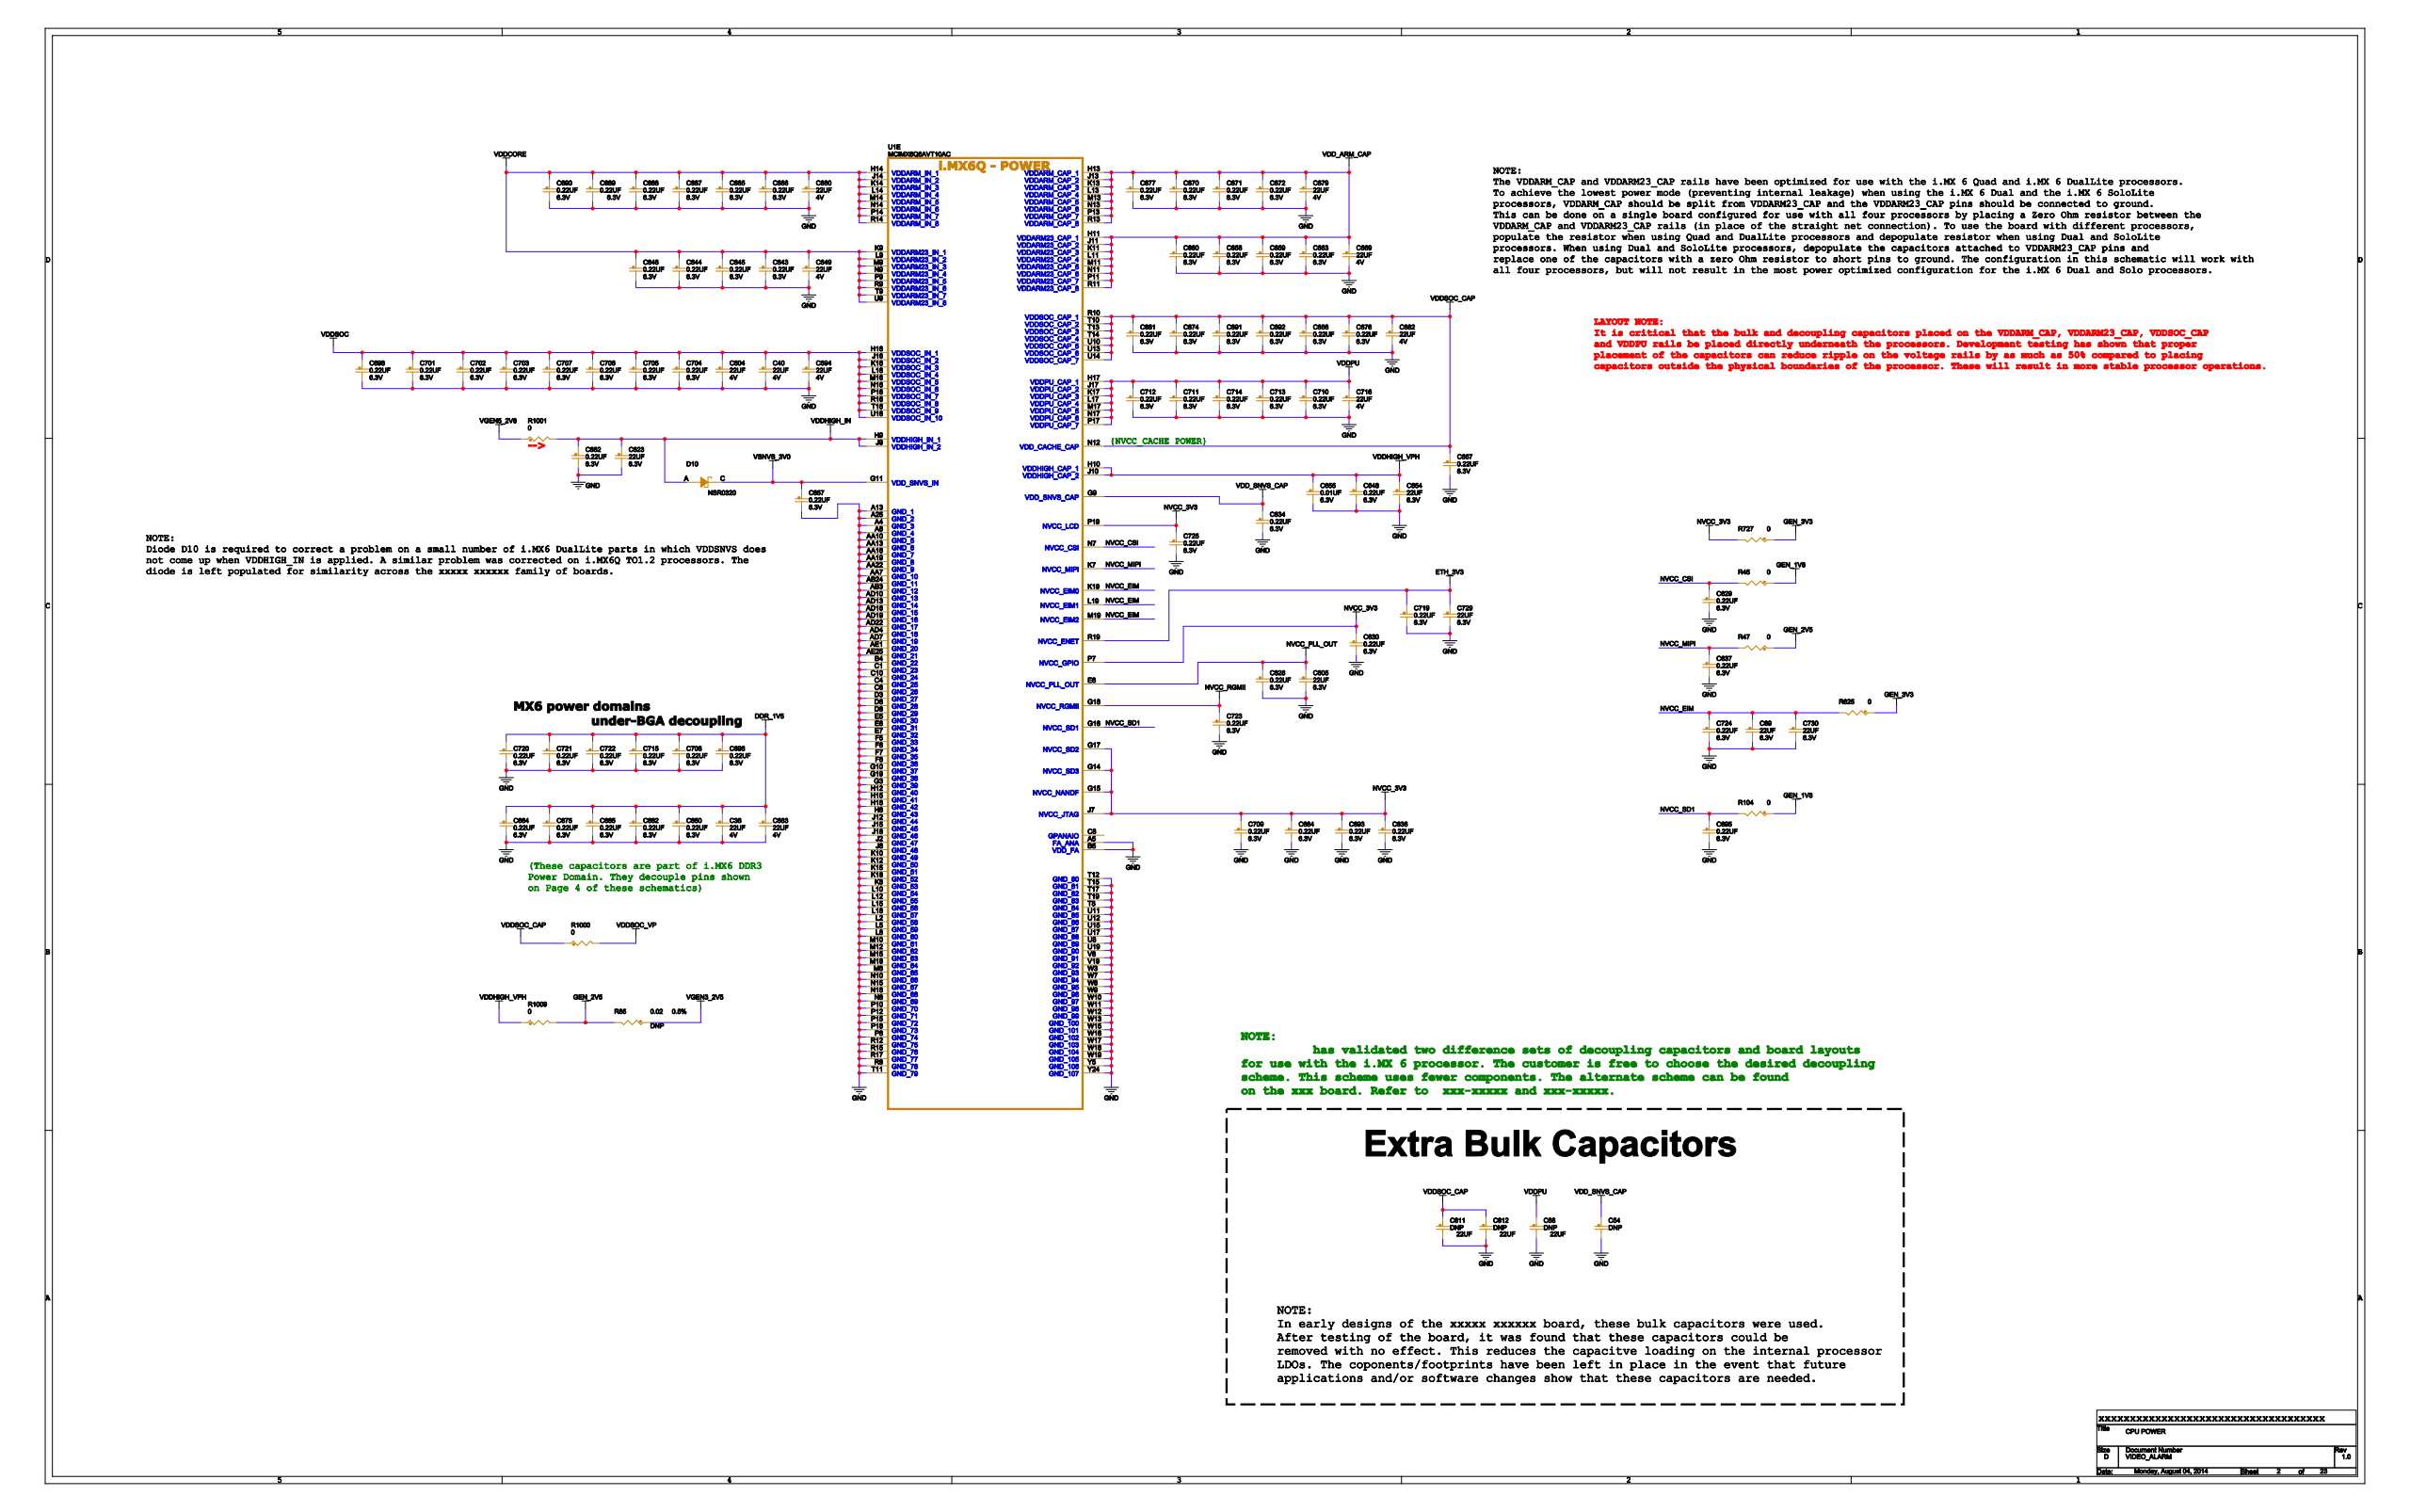Circuit board | Cadence Allegro | 994 parts | 728 nets | one sheet of the schematic
Parts on this sheet (reference | value | footprint):
C38 | 22UF | 0603_CC
C40 | 22UF | 0603_CC
C54 | 22UF | 0603_CC
C68 | 22UF | 0603_CC
C69 | 22UF | 0603_CC
C604 | 22UF | 0603_CC
C605 | 22UF | 0603_CC
C611 | 22UF | 0603_CC
C612 | 22UF | 0603_CC
C623 | 22UF | 0603_CC
C628 | 0.22UF | 0201_CC
C629 | 0.22UF | 0201_CC
C630 | 0.22UF | 0201_CC
C634 | 0.22UF | 0201_CC
C636 | 0.22UF | 0201_CC
C637 | 0.22UF | 0201_CC
C643 | 0.22UF | 0201_CC
C644 | 0.22UF | 0201_CC
C645 | 0.22UF | 0201_CC
C646 | 0.22UF | 0201_CC
C648 | 0.22UF | 0402_CC
C649 | 22UF | 0603_CC
C650 | 0.22UF | 0201_CC
C652 | 0.22UF | 0201_CC
C654 | 22UF | 0603_CC
C655 | 0.01UF | 0201_CC
C656 | 0.22UF | 0201_CC
C657 | 0.22UF | 0201_CC
C658 | 0.22UF | 0201_CC
C659 | 0.22UF | 0201_CC
C660 | 0.22UF | 0201_CC
C661 | 0.22UF | 0201_CC
C662 | 0.22UF | 0201_CC
C663 | 0.22UF | 0201_CC
C664 | 0.22UF | 0201_CC
C665 | 0.22UF | 0201_CC
C667 | 0.22UF | 0201_CC
C669 | 22UF | 0603_CC
C670 | 0.22UF | 0201_CC
C671 | 0.22UF | 0201_CC
C672 | 0.22UF | 0201_CC
C674 | 0.22UF | 0201_CC
C675 | 0.22UF | 0201_CC
C676 | 0.22UF | 0201_CC
C677 | 0.22UF | 0201_CC
C679 | 22UF | 0603_CC
C680 | 22UF | 0603_CC
C682 | 22UF | 0603_CC
C683 | 22UF | 0603_CC
C684 | 0.22UF | 0201_CC
C685 | 0.22UF | 0201_CC
C686 | 0.22UF | 0201_CC
C687 | 0.22UF | 0201_CC
C688 | 0.22UF | 0201_CC
C689 | 0.22UF | 0201_CC
C690 | 0.22UF | 0201_CC
C691 | 0.22UF | 0201_CC
C692 | 0.22UF | 0201_CC
C693 | 0.22UF | 0201_CC
C694 | 22UF | 0603_CC
C695 | 0.22UF | 0201_CC
C696 | 0.22UF | 0201_CC
C698 | 0.22UF | 0201_CC
C701 | 0.22UF | 0201_CC
C702 | 0.22UF | 0201_CC
C703 | 0.22UF | 0201_CC
C704 | 0.22UF | 0201_CC
C705 | 0.22UF | 0201_CC
C706 | 0.22UF | 0201_CC
C707 | 0.22UF | 0201_CC
C708 | 0.22UF | 0201_CC
C709 | 0.22UF | 0201_CC
C710 | 0.22UF | 0201_CC
C711 | 0.22UF | 0201_CC
C712 | 0.22UF | 0201_CC
C713 | 0.22UF | 0201_CC
C714 | 0.22UF | 0201_CC
C715 | 0.22UF | 0201_CC
C716 | 22UF | 0603_CC
C719 | 0.22UF | 0201_CC
C720 | 0.22UF | 0201_CC
C721 | 0.22UF | 0201_CC
C722 | 0.22UF | 0201_CC
C723 | 0.22UF | 0201_CC
C724 | 0.22UF | 0201_CC
C725 | 0.22UF | 0201_CC
C729 | 22UF | 0603_CC
C730 | 22UF | 0603_CC
D10 | NSR0320 | SOD323
J8 | 10029449-001RLF | HDMI
R45 | 0 | 0402_CC
R47 | 0 | 0402_CC
R85 | 0.02 | 0805_CC
R104 | 0 | 0402_CC
R625 | 0 | 0402_CC
R727 | 0 | 0402_CC
R1000 | 0 | 0805_CC
R1001 | 0 | 0805_CC
R1009 | 0 | 0805_CC
U1 | MCIMX6Q6AVT10AC | BGA624_0P8_21X21
U8 | MMPF0100F0EP | QFN56_0P5_8X8_EP4P5
U16 | CM2020 | TSSOP38_0P5_4P5X9P8
Nets of these parts (net: part-pin ...):
GND: C38-2 C40-2 C54-2 C68-2 C69-2 C604-2 C605-2 C611-2 C612-2 C623-2 C628-2 C629-2 C630-2 C634-2 C636-2 C637-2 C643-2 C644-2 C645-2 C646-2 C648-2 C649-2 C650-2 C652-2 C654-2 C655-2 C656-2 C657-2 C658-2 C659-2 C660-2 C661-2 C662-2 C663-2 C664-2 C665-2 C667-2 C669-2 C670-2 C671-2 C672-2 C674-2 C675-2 C676-2 C677-2 C679-2 C680-2 C682-2 C683-2 C684-2 C685-2 C686-2 C687-2 C688-2 C689-2 C690-2 C691-2 C692-2 C693-2 C694-2 C695-2 C696-2 C698-2 C701-2 C702-2 C703-2 C704-2 C705-2 C706-2 C707-2 C708-2 C709-2 C710-2 C711-2 C712-2 C713-2 C714-2 C715-2 C716-2 C719-2 C720-2 C721-2 C722-2 C723-2 C724-2 C725-2 C729-2 C730-2 J8-2 J8-5 U1-A4 U1-A5 U1-A8 U1-A13 U1-A25 U1-AA7 U1-AA10 U1-AA13 U1-AA16 U1-AA19 U1-AA22 U1-AB3 U1-AB24 U1-AD4 U1-AD7 U1-AD10 U1-AD13 U1-AD16 U1-AD19 U1-AD22 U1-AE1 U1-AE25 U1-B4 U1-B5 U1-C1 U1-C4 U1-C6 U1-C10 U1-D3 U1-D6 U1-D8 U1-E5 U1-E6 U1-E7 U1-F5 U1-F6 U1-F7 U1-F8 U1-G3 U1-G10 U1-G19 U1-H8 U1-H12 U1-H15 U1-H18 U1-J2 U1-J8 U1-J12 U1-J15 U1-J18 U1-K8 U1-K10 U1-K12 U1-K15 U1-K18 U1-L2 U1-L5 U1-L8 U1-L10 U1-L12 U1-L15 U1-L18 U1-M8 U1-M10 U1-M12 U1-M15 U1-M18 U1-N8 U1-N10 U1-N15 U1-N18 U1-P8 U1-P10 U1-P12 U1-P15 U1-P18 U1-R8 U1-R12 U1-R15 U1-R17 U1-T8 U1-T11 U1-T12 U1-T15 U1-T17 U1-T19 U1-U8 U1-U11 U1-U12 U1-U15 U1-U17 U1-U19 U1-V8 U1-V19 U1-W3 U1-W7 U1-W8 U1-W9 U1-W10 U1-W11 U1-W12 U1-W13 U1-W15 U1-W16 U1-W17 U1-W18 U1-W19 U1-Y5 U1-Y24 U8-5 U16-3 U16-5
GEN_3V3: R625-1 R727-1 U16-2
VGEN3_2V5: R85-1
VGEN5_2V8: R1001-1
DDR_1V5: C38-1 C650-1 C662-1 C664-1 C665-1 C675-1 C683-1 C696-1 C708-1 C715-1 C720-1 C721-1 C722-1
GEN_1V8: R45-1 R104-1
VDDCORE: C643-1 C644-1 C645-1 C646-1 C649-1 C680-1 C685-1 C686-1 C687-1 C688-1 C689-1 C690-1 U1-H14 U1-J14 U1-K9 U1-K14 U1-L9 U1-L14 U1-M9 U1-M14 U1-N9 U1-N14 U1-P9 U1-P14 U1-R9 U1-R14 U1-T9 U1-U9
VDDSOC: C40-1 C604-1 C694-1 C698-1 C701-1 C702-1 C703-1 C704-1 C705-1 C706-1 C707-1 U1-H16 U1-J16 U1-K16 U1-L16 U1-M16 U1-N16 U1-P16 U1-R16 U1-T16 U1-U16
VDDHIGH_VPH: C648-1 C654-1 C655-1 R1009-1 U1-H10 U1-J10
ETH_3V3: C719-1 C729-1 U1-R19
NVCC_RGMII: C723-1 U1-G18
VSNVS_3V0: C657-1 D10-C U1-G11
GPANAIO: U1-C8
NVCC_CSI: C629-1 R45-2 U1-N7
NVCC_EIM: C69-1 C724-1 C730-1 R625-2 U1-K19 U1-L19 U1-M19
NVCC_3V3: C630-1 C636-1 C684-1 C693-1 C709-1 C725-1 R727-2 U1-G14 U1-G15 U1-G17 U1-J7 U1-P7 U1-P19
NVCC_MIPI: C637-1 R47-2 U1-K7
NVCC_PLL_OUT: C605-1 C628-1 U1-E8
NVCC_SD1: C695-1 R104-2 U1-G16
VDD_ARM_CAP: C658-1 C659-1 C660-1 C663-1 C669-1 C670-1 C671-1 C672-1 C677-1 C679-1 U1-H11 U1-H13 U1-J11 U1-J13 U1-K11 U1-K13 U1-L11 U1-L13 U1-M11 U1-M13 U1-N11 U1-N13 U1-P11 U1-P13 U1-R11 U1-R13
VDDHIGH_IN: C623-1 C652-1 D10-A R1001-2 U1-H9 U1-J9
VDDPU: C68-1 C710-1 C711-1 C712-1 C713-1 C714-1 C716-1 U1-H17 U1-J17 U1-K17 U1-L17 U1-M17 U1-N17 U1-P17
VDDSOC_CAP: C611-1 C612-1 C656-1 C661-1 C667-1 C674-1 C676-1 C682-1 C691-1 C692-1 R1000-1 U1-N12 U1-R10 U1-T10 U1-T13 U1-T14 U1-U10 U1-U13 U1-U14
VDD_SNVS_CAP: C54-1 C634-1 U1-G9
GEN_2V5: R47-1 R85-2 R1009-2
VDDSOC_VP: R1000-2